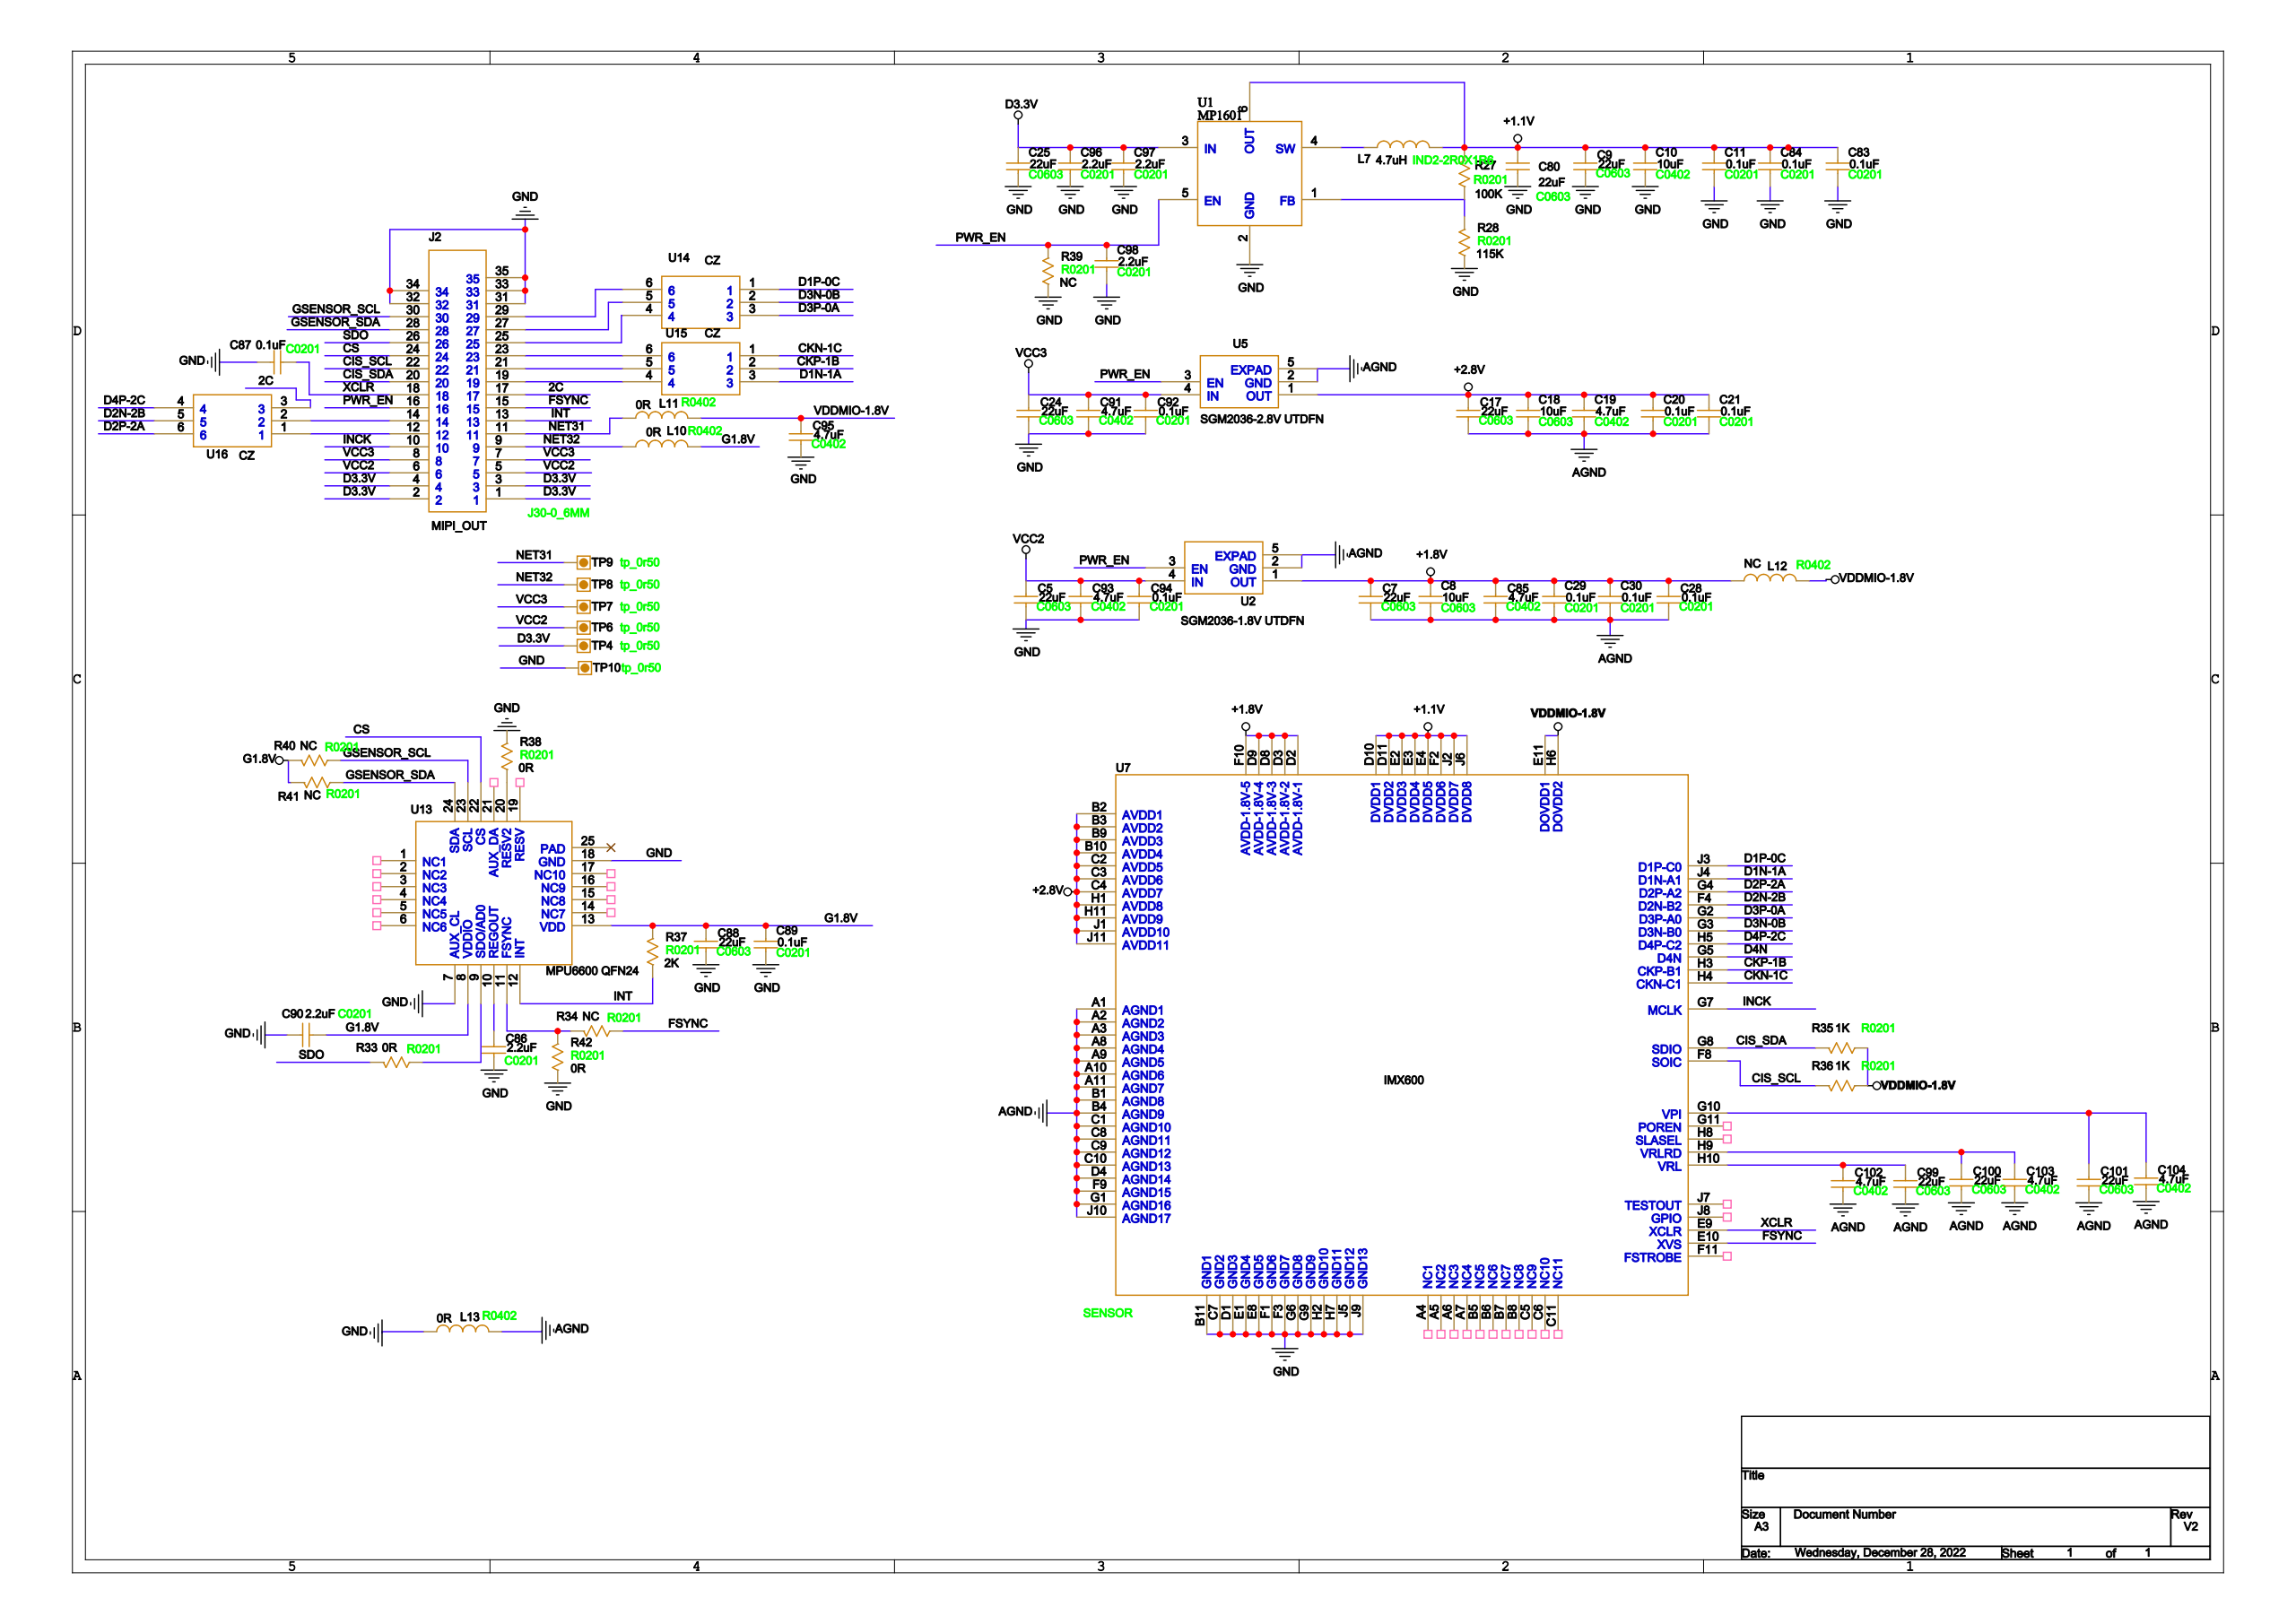Circuit board | Cadence Allegro | 71 parts | 51 nets
Bill of materials:
SYM_NAME,COMP_DEVICE_TYPE,COMP_VALUE,COMP_TOL,COMP_CLASS,REFDES
C0603,CAP_NP_C0603_22UF,22uF,,IC,C5
C0603,CAP_NP_C0603_22UF,22uF,,IC,C7
C0603,CAP_NP_C0603_10UF,10uF,,IC,C8
C0603,CAP_NP_C0603_22UF,22uF,,IC,C9
C0402,CAP_NP_C0402_10UF,10uF,,IC,C10
C0201,CAP_NP_C0201_0.1UF,0.1uF,,IC,C11
C0603,CAP_NP_C0603_22UF,22uF,,IC,C17
C0603,CAP_NP_C0603_10UF,10uF,,IC,C18
C0402,CAP_NP_C0402_4.7UF,4.7uF,,IC,C19
C0201,CAP_NP_C0201_0.1UF,0.1uF,,IC,C20
C0201,CAP_NP_C0201_0.1UF,0.1uF,,IC,C21
C0603,CAP_NP_C0603_22UF,22uF,,IC,C24
C0603,CAP_NP_C0603_22UF,22uF,,IC,C25
C0201,CAP_NP_C0201_0.1UF,0.1uF,,IC,C28
C0201,CAP_NP_C0201_0.1UF,0.1uF,,IC,C29
C0201,CAP_NP_C0201_0.1UF,0.1uF,,IC,C30
C0603,CAP_NP_C0603_22UF,22uF,,IC,C80
C0201,CAP_NP_C0201_0.1UF,0.1uF,,IC,C83
C0201,CAP_NP_C0201_0.1UF,0.1uF,,IC,C84
C0402,CAP_NP_C0402_4.7UF,4.7uF,,IC,C85
C0201,CAP_NP_C0201_2.2UF,2.2uF,,IC,C86
C0201,CAP_NP_C0201_0.1UF,0.1uF,,IC,C87
C0603,CAP_NP_C0603_22UF,22uF,,IC,C88
C0201,CAP_NP_C0201_0.1UF,0.1uF,,IC,C89
C0201,CAP_NP_C0201_2.2UF,2.2uF,,IC,C90
C0402,CAP_NP_C0402_4.7UF,4.7uF,,IC,C91
C0201,CAP_NP_C0201_0.1UF,0.1uF,,IC,C92
C0402,CAP_NP_C0402_4.7UF,4.7uF,,IC,C93
C0201,CAP_NP_C0201_0.1UF,0.1uF,,IC,C94
C0402,CAP_NP_C0402_4.7UF,4.7uF,,IC,C95
C0201,CAP_NP_C0201_2.2UF,2.2uF,,IC,C96
C0201,CAP_NP_C0201_2.2UF,2.2uF,,IC,C97
C0201,CAP_NP_C0201_2.2UF,2.2uF,,IC,C98
C0603,CAP_NP_C0603_22UF,22uF,,IC,C99
C0603,CAP_NP_C0603_22UF,22uF,,IC,C100
C0603,CAP_NP_C0603_22UF,22uF,,IC,C101
C0402,CAP_NP_C0402_4.7UF,4.7uF,,IC,C102
C0402,CAP_NP_C0402_4.7UF,4.7uF,,IC,C103
C0402,CAP_NP_C0402_4.7UF,4.7uF,,IC,C104
J30-0_6MM,CON4_7_J30-0_6MM_MIPI_OUT,MIPI_OUT,,IC,J2
IND2-2R0X1R6,L_SMD_IND2-2R0X1R6_4.7UH,4.7uH,,IC,L7
R0402,INDUCTOR_R0402_0R,0R,,IC,L10
R0402,INDUCTOR_R0402_0R,0R,,IC,L11
R0402,INDUCTOR_R0402_NC,NC,,IC,L12
R0402,INDUCTOR_R0402_0R,0R,,IC,L13
R0201,R_R0201_100K,100K,,IC,R27
R0201,R_R0201_115K,115K,,IC,R28
R0201,R_R0201_0R,0R,,IC,R33
R0201,R_R0201_NC,NC,,IC,R34
R0201,R_R0201_1K,1K,,IC,R35
R0201,R_R0201_1K,1K,,IC,R36
R0201,R_R0201_2K,2K,,IC,R37
R0201,R_R0201_0R,0R,,IC,R38
R0201,R_R0201_NC,NC,,IC,R39
R0201,R_R0201_NC,NC,,IC,R40
R0201,R_R0201_NC,NC,,IC,R41
R0201,R_R0201_0R,0R,,IC,R42
TP_0R50,TESTPOINT_0_TP_0R50_TESTPOINT,TestPoint,,IC,TP4
TP_0R50,TESTPOINT_0_TP_0R50_TESTPOINT,TestPoint,,IC,TP6
TP_0R50,TESTPOINT_0_TP_0R50_TESTPOINT,TestPoint,,IC,TP7
TP_0R50,TESTPOINT_0_TP_0R50_TESTPOINT,TestPoint,,IC,TP8
TP_0R50,TESTPOINT_0_TP_0R50_TESTPOINT,TestPoint,,IC,TP9
TP_0R50,TESTPOINT_0_TP_0R50_TESTPOINT,TestPoint,,IC,TP10
UTDFN_1X1-4L,SGM2036_UTDFN_UTDFN_1X1-4L_SGM2,SGM2036-1.8V UTDFN,,IC,U2
UTDFN_1X1-4L,SGM2036_UTDFN_UTDFN_1X1-4L_SG_1,SGM2036-2.8V UTDFN,,IC,U5
SENSOR,AR0230_15_SENSOR_IMX600,IMX600,,IC,U7
SOT563_1R5X1R2,M3406_4_SOT563_1R5X1R2_MP1601,MP1601,,IC,U9
MCU_QFN20_S120,MCU_5_MCU_QFN20_S120_MPU6600 QF,MPU6600 QFN24,,IC,U13
0201_3,SGM2036_UTDFN_0_0201_3_CZ,CZ,,DISCRETE,U14
0201_3,SGM2036_UTDFN_0_0201_3_CZ,CZ,,DISCRETE,U15
0201_3,SGM2036_UTDFN_0_0201_3_CZ,CZ,,DISCRETE,U16
Netlist (net: part-pin ...):
GND: C5-2 C9-2 C10-2 C11-2 C24-2 C25-2 C80-2 C83-2 C84-2 C86-2 C87-2 C88-2 C89-2 C90-1 C91-2 C92-2 C93-2 C94-2 C95-2 C96-2 C97-2 C98-2 J2-31 J2-32 J2-33 J2-34 J2-35 L13-1 R28-1 R38-2 R39-1 R42-1 TP10-1 U7-B11 U7-C7 U7-D1 U7-E1 U7-E8 U7-F1 U7-F3 U7-G6 U7-G9 U7-H2 U7-H7 U7-J5 U7-J9 U9-2 U13-7 U13-18
CS: J2-24 U13-22
N21679881: R34-2 R42-2 U13-11
INT: J2-13 R37-1 U13-12
N21675405: C86-1 U13-10
N2167319219: R38-1 U13-20
GSENSOR_SCL: J2-30 R40-1 U13-23
GSENSOR_SDA: J2-28 R41-1 U13-24
N21679670: R33-1 U13-9
G1.8V: C88-1 C89-1 C90-2 L10-2 R37-2 R40-2 R41-2 U13-8 U13-13
+1.1V: C9-1 C10-1 C11-1 C80-1 C83-1 C84-1 L7-2 R27-2 U7-D10 U7-D11 U7-E2 U7-E3 U7-E4 U7-F2 U7-J2 U7-J6 U9-6
+2.8V: C17-1 C18-1 C19-1 C20-1 C21-1 U5-1 U7-B2 U7-B3 U7-B9 U7-B10 U7-C2 U7-C3 U7-C4 U7-H1 U7-H11 U7-J1 U7-J11
AGND: C7-2 C8-2 C17-2 C18-2 C19-2 C20-2 C21-2 C28-2 C29-2 C30-2 C85-2 C99-2 C100-2 C101-2 C102-2 C103-2 C104-2 L13-2 U2-2 U2-5 U5-2 U5-5 U7-A1 U7-A2 U7-A3 U7-A8 U7-A9 U7-A10 U7-A11 U7-B1 U7-B4 U7-C1 U7-C8 U7-C9 U7-C10 U7-D4 U7-F9 U7-G1 U7-J10
+1.8V: C7-1 C8-1 C28-1 C29-1 C30-1 C85-1 L12-1 U2-1 U7-D2 U7-D3 U7-D8 U7-D9 U7-F10
D3.3V: C25-1 C96-1 C97-1 J2-1 J2-2 J2-3 J2-4 TP4-1 U9-3
INCK: J2-10 U7-G7
NET31: J2-11 L11-1 TP9-1
N21668905: J2-12 U16-1
N21668842: J2-14 U16-2
FSYNC: J2-15 R34-1 U7-E10
PWR_EN: C98-1 J2-16 R39-2 U2-3 U5-3 U9-5
2C: J2-17 U16-3
XCLR: C87-1 J2-18 U7-E9
N21679792: J2-19 U15-4
CIS_SDA: J2-20 R35-2 U7-G8
N21668777: J2-21 U15-5
CIS_SCL: J2-22 R36-2 U7-F8
N21668783: J2-23 U15-6
N21668792: J2-25 U14-4
SDO: J2-26 R33-2
N21668789: J2-27 U14-5
N21668786: J2-29 U14-6
VCC2: C5-1 C93-1 C94-1 J2-5 J2-6 TP6-1 U2-4
VCC3: C24-1 C91-1 C92-1 J2-7 J2-8 TP7-1 U5-4
NET32: J2-9 L10-1 TP8-1
VDDMIO-1.8V: C95-1 L11-2 L12-2 R35-1 R36-1 U7-E11 U7-H6
D1P-0C: U7-J3 U14-1
D3N-0B: U7-G3 U14-2
D3P-0A: U7-G2 U14-3
CKN-1C: U7-H4 U15-1
CKP-1B: U7-H3 U15-2
D1N-1A: U7-J4 U15-3
D4P-2C: U7-H5 U16-4
D2N-2B: U7-F4 U16-5
D2P-2A: U7-G4 U16-6
D4N: U7-G5
N21690320: C101-1 C104-1 U7-G10
N21688066: C99-1 C102-1 U7-H10
N21688059: C100-1 C103-1 U7-H9
N21658763: L7-1 U9-4
N21658749: R27-1 R28-2 U9-1